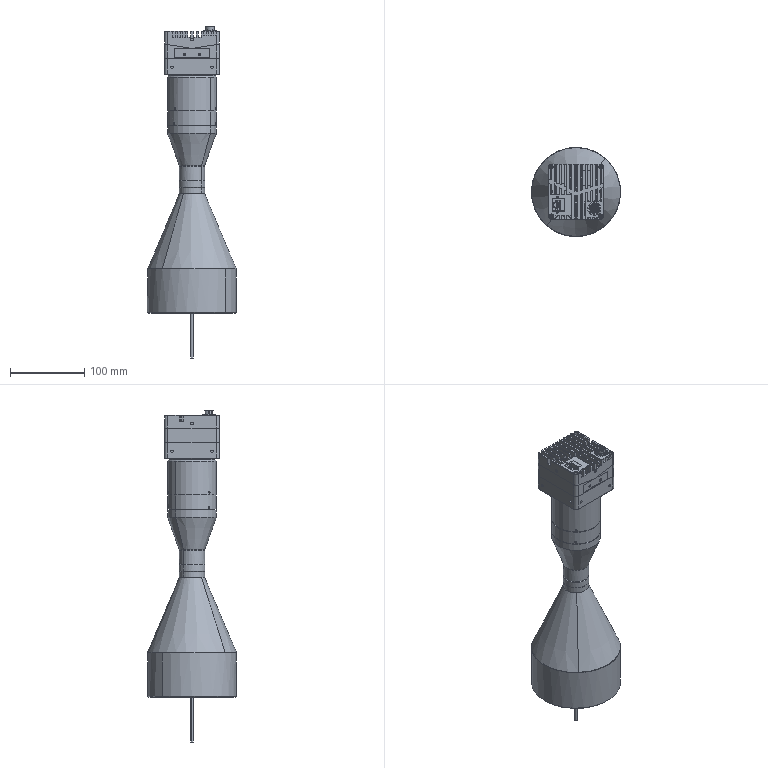Part | SolidWorks | 25 solids | 1904 faces | box 120 x 120 x 447.19 mm | volume 1943055 mm3 | plane 1183 | cylinder 603 | cone 80 | spline 34 | torus 4 | commonest cylinder face diameters 2 x83 0.6 x56 2.5 x44 0.5 x36 0.4 x32 3.3 x32